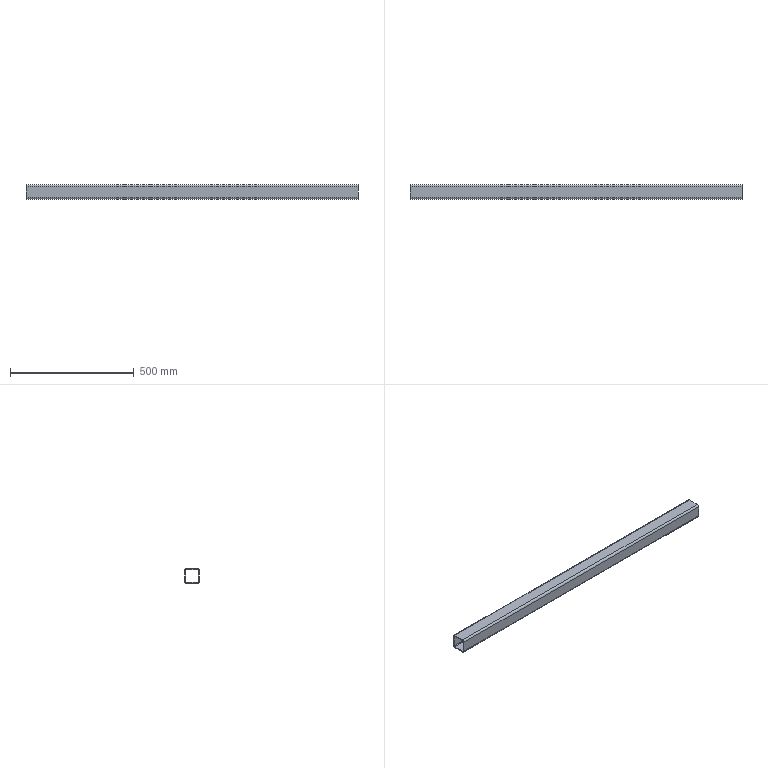Part | SolidWorks | features BaseBody 1 | 1 solid | 18 faces | box 1340 x 60 x 60 mm | volume 1145427 mm3 | plane 10 | cylinder 8 | commonest cylinder face diameters 8 x4 16 x4
STEP:
#1=CARTESIAN_POINT('',(-640.,44.,504.));
#2=VERTEX_POINT('',#1);
#3=CARTESIAN_POINT('',(-640.,0.,504.));
#4=VERTEX_POINT('',#3);
#5=CARTESIAN_POINT('',(-640.,44.,504.));
#6=DIRECTION('',(0.,-1.,0.));
#7=VECTOR('',#6,1000.);
#8=LINE('',#5,#7);
#9=EDGE_CURVE('',#2,#4,#8,.T.);
#10=ORIENTED_EDGE('',*,*,#9,.T.);
#11=CARTESIAN_POINT('',(700.,0.,504.));
#12=VERTEX_POINT('',#11);
#13=CARTESIAN_POINT('',(-670.,0.,504.));
#14=DIRECTION('',(1.,0.,0.));
#15=VECTOR('',#14,1000.);
#16=LINE('',#13,#15);
#17=EDGE_CURVE('',#4,#12,#16,.T.);
#18=ORIENTED_EDGE('',*,*,#17,.T.);
#19=CARTESIAN_POINT('',(700.,44.,504.));
#20=VERTEX_POINT('',#19);
#21=CARTESIAN_POINT('',(700.,44.,504.));
#22=DIRECTION('',(0.,1.,0.));
#23=VECTOR('',#22,1000.);
#24=LINE('',#21,#23);
#25=EDGE_CURVE('',#12,#20,#24,.T.);
#26=ORIENTED_EDGE('',*,*,#25,.T.);
#27=CARTESIAN_POINT('',(-670.,44.,504.));
#28=DIRECTION('',(-1.,0.,0.));
#29=VECTOR('',#28,1000.);
#30=LINE('',#27,#29);
#31=EDGE_CURVE('',#20,#2,#30,.T.);
#32=ORIENTED_EDGE('',*,*,#31,.T.);
#33=EDGE_LOOP('',(#10,#18,#26,#32));
#34=FACE_OUTER_BOUND('',#33,.T.);
#35=CARTESIAN_POINT('',(-670.,44.,504.));
#36=DIRECTION('',(0.,0.,1.));
#37=DIRECTION('',(1.,0.,0.));
#38=AXIS2_PLACEMENT_3D('',#35,#36,#37);
#39=PLANE('',#38);
#40=ADVANCED_FACE('',(#34),#39,.T.);
#41=ORIENTED_EDGE('',*,*,#17,.F.);
#42=CARTESIAN_POINT('',(-640.,-4.,508.));
#43=VERTEX_POINT('',#42);
#44=CARTESIAN_POINT('',(-640.,0.,508.));
#45=DIRECTION('',(1.,0.,0.));
#46=DIRECTION('',(0.,0.,-1.));
#47=AXIS2_PLACEMENT_3D('',#44,#45,#46);
#48=CIRCLE('',#47,4.);
#49=EDGE_CURVE('',#43,#4,#48,.T.);
#50=ORIENTED_EDGE('',*,*,#49,.F.);
#51=CARTESIAN_POINT('',(700.,-4.,508.));
#52=VERTEX_POINT('',#51);
#53=CARTESIAN_POINT('',(-670.,-4.,508.));
#54=DIRECTION('',(-1.,0.,0.));
#55=VECTOR('',#54,1000.);
#56=LINE('',#53,#55);
#57=EDGE_CURVE('',#52,#43,#56,.T.);
#58=ORIENTED_EDGE('',*,*,#57,.F.);
#59=CARTESIAN_POINT('',(700.,0.,508.));
#60=DIRECTION('',(-1.,0.,0.));
#61=DIRECTION('',(0.,0.,-1.));
#62=AXIS2_PLACEMENT_3D('',#59,#60,#61);
#63=CIRCLE('',#62,4.);
#64=EDGE_CURVE('',#12,#52,#63,.T.);
#65=ORIENTED_EDGE('',*,*,#64,.F.);
#66=EDGE_LOOP('',(#41,#50,#58,#65));
#67=FACE_OUTER_BOUND('',#66,.T.);
#68=CARTESIAN_POINT('',(-670.,0.,508.));
#69=DIRECTION('',(1.,0.,0.));
#70=DIRECTION('',(0.,0.,-1.));
#71=AXIS2_PLACEMENT_3D('',#68,#69,#70);
#72=CYLINDRICAL_SURFACE('',#71,4.);
#73=ADVANCED_FACE('',(#67),#72,.F.);
#74=ORIENTED_EDGE('',*,*,#49,.T.);
#75=ORIENTED_EDGE('',*,*,#9,.F.);
#76=CARTESIAN_POINT('',(-640.,48.,508.));
#77=VERTEX_POINT('',#76);
#78=CARTESIAN_POINT('',(-640.,44.,508.));
#79=DIRECTION('',(1.,0.,0.));
#80=DIRECTION('',(0.,0.,-1.));
#81=AXIS2_PLACEMENT_3D('',#78,#79,#80);
#82=CIRCLE('',#81,4.);
#83=EDGE_CURVE('',#2,#77,#82,.T.);
#84=ORIENTED_EDGE('',*,*,#83,.T.);
#85=CARTESIAN_POINT('',(-640.,48.,552.));
#86=VERTEX_POINT('',#85);
#87=CARTESIAN_POINT('',(-640.,48.,508.));
#88=DIRECTION('',(0.,0.,1.));
#89=VECTOR('',#88,1000.);
#90=LINE('',#87,#89);
#91=EDGE_CURVE('',#77,#86,#90,.T.);
#92=ORIENTED_EDGE('',*,*,#91,.T.);
#93=CARTESIAN_POINT('',(-640.,44.,556.));
#94=VERTEX_POINT('',#93);
#95=CARTESIAN_POINT('',(-640.,44.,552.));
#96=DIRECTION('',(1.,0.,0.));
#97=DIRECTION('',(0.,0.,-1.));
#98=AXIS2_PLACEMENT_3D('',#95,#96,#97);
#99=CIRCLE('',#98,4.);
#100=EDGE_CURVE('',#86,#94,#99,.T.);
#101=ORIENTED_EDGE('',*,*,#100,.T.);
#102=CARTESIAN_POINT('',(-640.,0.,556.));
#103=VERTEX_POINT('',#102);
#104=CARTESIAN_POINT('',(-640.,1242.,556.));
#105=DIRECTION('',(0.,-1.,0.));
#106=VECTOR('',#105,1000.);
#107=LINE('',#104,#106);
#108=EDGE_CURVE('',#94,#103,#107,.T.);
#109=ORIENTED_EDGE('',*,*,#108,.T.);
#110=CARTESIAN_POINT('',(-640.,-4.,552.));
#111=VERTEX_POINT('',#110);
#112=CARTESIAN_POINT('',(-640.,0.,552.));
#113=DIRECTION('',(1.,0.,0.));
#114=DIRECTION('',(0.,0.,-1.));
#115=AXIS2_PLACEMENT_3D('',#112,#113,#114);
#116=CIRCLE('',#115,4.);
#117=EDGE_CURVE('',#103,#111,#116,.T.);
#118=ORIENTED_EDGE('',*,*,#117,.T.);
#119=CARTESIAN_POINT('',(-640.,-4.,508.));
#120=DIRECTION('',(0.,0.,-1.));
#121=VECTOR('',#120,1000.);
#122=LINE('',#119,#121);
#123=EDGE_CURVE('',#111,#43,#122,.T.);
#124=ORIENTED_EDGE('',*,*,#123,.T.);
#125=EDGE_LOOP('',(#74,#75,#84,#92,#101,#109,#118,#124));
#126=FACE_BOUND('',#125,.T.);
#127=CARTESIAN_POINT('',(-640.,44.,500.));
#128=VERTEX_POINT('',#127);
#129=CARTESIAN_POINT('',(-640.,0.,500.));
#130=VERTEX_POINT('',#129);
#131=CARTESIAN_POINT('',(-640.,1242.,500.));
#132=DIRECTION('',(0.,-1.,0.));
#133=VECTOR('',#132,1000.);
#134=LINE('',#131,#133);
#135=EDGE_CURVE('',#128,#130,#134,.T.);
#136=ORIENTED_EDGE('',*,*,#135,.T.);
#137=CARTESIAN_POINT('',(-640.,-8.,508.));
#138=VERTEX_POINT('',#137);
#139=CARTESIAN_POINT('',(-640.,0.,508.));
#140=DIRECTION('',(-1.,0.,0.));
#141=DIRECTION('',(0.,0.,-1.));
#142=AXIS2_PLACEMENT_3D('',#139,#140,#141);
#143=CIRCLE('',#142,8.);
#144=EDGE_CURVE('',#130,#138,#143,.T.);
#145=ORIENTED_EDGE('',*,*,#144,.T.);
#146=CARTESIAN_POINT('',(-640.,-8.,552.));
#147=VERTEX_POINT('',#146);
#148=CARTESIAN_POINT('',(-640.,-8.,508.));
#149=DIRECTION('',(0.,0.,1.));
#150=VECTOR('',#149,1000.);
#151=LINE('',#148,#150);
#152=EDGE_CURVE('',#138,#147,#151,.T.);
#153=ORIENTED_EDGE('',*,*,#152,.T.);
#154=CARTESIAN_POINT('',(-640.,0.,560.));
#155=VERTEX_POINT('',#154);
#156=CARTESIAN_POINT('',(-640.,0.,552.));
#157=DIRECTION('',(-1.,0.,0.));
#158=DIRECTION('',(0.,0.,-1.));
#159=AXIS2_PLACEMENT_3D('',#156,#157,#158);
#160=CIRCLE('',#159,8.);
#161=EDGE_CURVE('',#147,#155,#160,.T.);
#162=ORIENTED_EDGE('',*,*,#161,.T.);
#163=CARTESIAN_POINT('',(-640.,44.,560.));
#164=VERTEX_POINT('',#163);
#165=CARTESIAN_POINT('',(-640.,1242.,560.));
#166=DIRECTION('',(0.,1.,0.));
#167=VECTOR('',#166,1000.);
#168=LINE('',#165,#167);
#169=EDGE_CURVE('',#155,#164,#168,.T.);
#170=ORIENTED_EDGE('',*,*,#169,.T.);
#171=CARTESIAN_POINT('',(-640.,52.,552.));
#172=VERTEX_POINT('',#171);
#173=CARTESIAN_POINT('',(-640.,44.,552.));
#174=DIRECTION('',(-1.,0.,0.));
#175=DIRECTION('',(0.,0.,-1.));
#176=AXIS2_PLACEMENT_3D('',#173,#174,#175);
#177=CIRCLE('',#176,8.);
#178=EDGE_CURVE('',#164,#172,#177,.T.);
#179=ORIENTED_EDGE('',*,*,#178,.T.);
#180=CARTESIAN_POINT('',(-640.,52.,508.));
#181=VERTEX_POINT('',#180);
#182=CARTESIAN_POINT('',(-640.,52.,508.));
#183=DIRECTION('',(0.,0.,-1.));
#184=VECTOR('',#183,1000.);
#185=LINE('',#182,#184);
#186=EDGE_CURVE('',#172,#181,#185,.T.);
#187=ORIENTED_EDGE('',*,*,#186,.T.);
#188=CARTESIAN_POINT('',(-640.,44.,508.));
#189=DIRECTION('',(-1.,0.,0.));
#190=DIRECTION('',(0.,0.,-1.));
#191=AXIS2_PLACEMENT_3D('',#188,#189,#190);
#192=CIRCLE('',#191,8.);
#193=EDGE_CURVE('',#181,#128,#192,.T.);
#194=ORIENTED_EDGE('',*,*,#193,.T.);
#195=EDGE_LOOP('',(#136,#145,#153,#162,#170,#179,#187,#194));
#196=FACE_OUTER_BOUND('',#195,.T.);
#197=CARTESIAN_POINT('',(-640.,1242.,508.));
#198=DIRECTION('',(-1.,0.,0.));
#199=DIRECTION('',(0.,0.,1.));
#200=AXIS2_PLACEMENT_3D('',#197,#198,#199);
#201=PLANE('',#200);
#202=ADVANCED_FACE('',(#126,#196),#201,.T.);
#203=CARTESIAN_POINT('',(700.,48.,508.));
#204=VERTEX_POINT('',#203);
#205=CARTESIAN_POINT('',(-670.,48.,508.));
#206=DIRECTION('',(1.,0.,0.));
#207=VECTOR('',#206,1000.);
#208=LINE('',#205,#207);
#209=EDGE_CURVE('',#77,#204,#208,.T.);
#210=ORIENTED_EDGE('',*,*,#209,.F.);
#211=ORIENTED_EDGE('',*,*,#83,.F.);
#212=ORIENTED_EDGE('',*,*,#31,.F.);
#213=CARTESIAN_POINT('',(700.,44.,508.));
#214=DIRECTION('',(-1.,0.,0.));
#215=DIRECTION('',(0.,0.,-1.));
#216=AXIS2_PLACEMENT_3D('',#213,#214,#215);
#217=CIRCLE('',#216,4.);
#218=EDGE_CURVE('',#204,#20,#217,.T.);
#219=ORIENTED_EDGE('',*,*,#218,.F.);
#220=EDGE_LOOP('',(#210,#211,#212,#219));
#221=FACE_OUTER_BOUND('',#220,.T.);
#222=CARTESIAN_POINT('',(-670.,44.,508.));
#223=DIRECTION('',(1.,0.,0.));
#224=DIRECTION('',(0.,0.,-1.));
#225=AXIS2_PLACEMENT_3D('',#222,#223,#224);
#226=CYLINDRICAL_SURFACE('',#225,4.);
#227=ADVANCED_FACE('',(#221),#226,.F.);
#228=ORIENTED_EDGE('',*,*,#25,.F.);
#229=ORIENTED_EDGE('',*,*,#64,.T.);
#230=CARTESIAN_POINT('',(700.,-4.,552.));
#231=VERTEX_POINT('',#230);
#232=CARTESIAN_POINT('',(700.,-4.,530.));
#233=DIRECTION('',(0.,0.,1.));
#234=VECTOR('',#233,1000.);
#235=LINE('',#232,#234);
#236=EDGE_CURVE('',#52,#231,#235,.T.);
#237=ORIENTED_EDGE('',*,*,#236,.T.);
#238=CARTESIAN_POINT('',(700.,0.,556.));
#239=VERTEX_POINT('',#238);
#240=CARTESIAN_POINT('',(700.,0.,552.));
#241=DIRECTION('',(-1.,0.,0.));
#242=DIRECTION('',(0.,0.,-1.));
#243=AXIS2_PLACEMENT_3D('',#240,#241,#242);
#244=CIRCLE('',#243,4.);
#245=EDGE_CURVE('',#231,#239,#244,.T.);
#246=ORIENTED_EDGE('',*,*,#245,.T.);
#247=CARTESIAN_POINT('',(700.,44.,556.));
#248=VERTEX_POINT('',#247);
#249=CARTESIAN_POINT('',(700.,52.,556.));
#250=DIRECTION('',(0.,1.,0.));
#251=VECTOR('',#250,1000.);
#252=LINE('',#249,#251);
#253=EDGE_CURVE('',#239,#248,#252,.T.);
#254=ORIENTED_EDGE('',*,*,#253,.T.);
#255=CARTESIAN_POINT('',(700.,48.,552.));
#256=VERTEX_POINT('',#255);
#257=CARTESIAN_POINT('',(700.,44.,552.));
#258=DIRECTION('',(-1.,0.,0.));
#259=DIRECTION('',(0.,0.,-1.));
#260=AXIS2_PLACEMENT_3D('',#257,#258,#259);
#261=CIRCLE('',#260,4.);
#262=EDGE_CURVE('',#248,#256,#261,.T.);
#263=ORIENTED_EDGE('',*,*,#262,.T.);
#264=CARTESIAN_POINT('',(700.,48.,530.));
#265=DIRECTION('',(0.,0.,-1.));
#266=VECTOR('',#265,1000.);
#267=LINE('',#264,#266);
#268=EDGE_CURVE('',#256,#204,#267,.T.);
#269=ORIENTED_EDGE('',*,*,#268,.T.);
#270=ORIENTED_EDGE('',*,*,#218,.T.);
#271=EDGE_LOOP('',(#228,#229,#237,#246,#254,#263,#269,#270));
#272=FACE_BOUND('',#271,.T.);
#273=CARTESIAN_POINT('',(700.,-8.,508.));
#274=VERTEX_POINT('',#273);
#275=CARTESIAN_POINT('',(700.,0.,500.));
#276=VERTEX_POINT('',#275);
#277=CARTESIAN_POINT('',(700.,0.,508.));
#278=DIRECTION('',(1.,0.,0.));
#279=DIRECTION('',(0.,0.,-1.));
#280=AXIS2_PLACEMENT_3D('',#277,#278,#279);
#281=CIRCLE('',#280,8.);
#282=EDGE_CURVE('',#274,#276,#281,.T.);
#283=ORIENTED_EDGE('',*,*,#282,.T.);
#284=CARTESIAN_POINT('',(700.,44.,500.));
#285=VERTEX_POINT('',#284);
#286=CARTESIAN_POINT('',(700.,52.,500.));
#287=DIRECTION('',(0.,1.,0.));
#288=VECTOR('',#287,1000.);
#289=LINE('',#286,#288);
#290=EDGE_CURVE('',#276,#285,#289,.T.);
#291=ORIENTED_EDGE('',*,*,#290,.T.);
#292=CARTESIAN_POINT('',(700.,52.,508.));
#293=VERTEX_POINT('',#292);
#294=CARTESIAN_POINT('',(700.,44.,508.));
#295=DIRECTION('',(1.,0.,0.));
#296=DIRECTION('',(0.,0.,-1.));
#297=AXIS2_PLACEMENT_3D('',#294,#295,#296);
#298=CIRCLE('',#297,8.);
#299=EDGE_CURVE('',#285,#293,#298,.T.);
#300=ORIENTED_EDGE('',*,*,#299,.T.);
#301=CARTESIAN_POINT('',(700.,52.,552.));
#302=VERTEX_POINT('',#301);
#303=CARTESIAN_POINT('',(700.,52.,530.));
#304=DIRECTION('',(0.,0.,1.));
#305=VECTOR('',#304,1000.);
#306=LINE('',#303,#305);
#307=EDGE_CURVE('',#293,#302,#306,.T.);
#308=ORIENTED_EDGE('',*,*,#307,.T.);
#309=CARTESIAN_POINT('',(700.,44.,560.));
#310=VERTEX_POINT('',#309);
#311=CARTESIAN_POINT('',(700.,44.,552.));
#312=DIRECTION('',(1.,0.,0.));
#313=DIRECTION('',(0.,0.,-1.));
#314=AXIS2_PLACEMENT_3D('',#311,#312,#313);
#315=CIRCLE('',#314,8.);
#316=EDGE_CURVE('',#302,#310,#315,.T.);
#317=ORIENTED_EDGE('',*,*,#316,.T.);
#318=CARTESIAN_POINT('',(700.,0.,560.));
#319=VERTEX_POINT('',#318);
#320=CARTESIAN_POINT('',(700.,52.,560.));
#321=DIRECTION('',(0.,-1.,0.));
#322=VECTOR('',#321,1000.);
#323=LINE('',#320,#322);
#324=EDGE_CURVE('',#310,#319,#323,.T.);
#325=ORIENTED_EDGE('',*,*,#324,.T.);
#326=CARTESIAN_POINT('',(700.,-8.,552.));
#327=VERTEX_POINT('',#326);
#328=CARTESIAN_POINT('',(700.,0.,552.));
#329=DIRECTION('',(1.,0.,0.));
#330=DIRECTION('',(0.,0.,-1.));
#331=AXIS2_PLACEMENT_3D('',#328,#329,#330);
#332=CIRCLE('',#331,8.);
#333=EDGE_CURVE('',#319,#327,#332,.T.);
#334=ORIENTED_EDGE('',*,*,#333,.T.);
#335=CARTESIAN_POINT('',(700.,-8.,530.));
#336=DIRECTION('',(0.,0.,-1.));
#337=VECTOR('',#336,1000.);
#338=LINE('',#335,#337);
#339=EDGE_CURVE('',#327,#274,#338,.T.);
#340=ORIENTED_EDGE('',*,*,#339,.T.);
#341=EDGE_LOOP('',(#283,#291,#300,#308,#317,#325,#334,#340));
#342=FACE_OUTER_BOUND('',#341,.T.);
#343=CARTESIAN_POINT('',(700.,52.,530.));
#344=DIRECTION('',(1.,0.,0.));
#345=DIRECTION('',(0.,0.,-1.));
#346=AXIS2_PLACEMENT_3D('',#343,#344,#345);
#347=PLANE('',#346);
#348=ADVANCED_FACE('',(#272,#342),#347,.T.);
#349=ORIENTED_EDGE('',*,*,#123,.F.);
#350=CARTESIAN_POINT('',(-670.,-4.,552.));
#351=DIRECTION('',(1.,0.,0.));
#352=VECTOR('',#351,1000.);
#353=LINE('',#350,#352);
#354=EDGE_CURVE('',#111,#231,#353,.T.);
#355=ORIENTED_EDGE('',*,*,#354,.T.);
#356=ORIENTED_EDGE('',*,*,#236,.F.);
#357=ORIENTED_EDGE('',*,*,#57,.T.);
#358=EDGE_LOOP('',(#349,#355,#356,#357));
#359=FACE_OUTER_BOUND('',#358,.T.);
#360=CARTESIAN_POINT('',(-670.,-4.,552.));
#361=DIRECTION('',(0.,1.,0.));
#362=DIRECTION('',(0.,0.,1.));
#363=AXIS2_PLACEMENT_3D('',#360,#361,#362);
#364=PLANE('',#363);
#365=ADVANCED_FACE('',(#359),#364,.T.);
#366=ORIENTED_EDGE('',*,*,#354,.F.);
#367=ORIENTED_EDGE('',*,*,#117,.F.);
#368=CARTESIAN_POINT('',(-670.,0.,556.));
#369=DIRECTION('',(-1.,0.,0.));
#370=VECTOR('',#369,1000.);
#371=LINE('',#368,#370);
#372=EDGE_CURVE('',#239,#103,#371,.T.);
#373=ORIENTED_EDGE('',*,*,#372,.F.);
#374=ORIENTED_EDGE('',*,*,#245,.F.);
#375=EDGE_LOOP('',(#366,#367,#373,#374));
#376=FACE_OUTER_BOUND('',#375,.T.);
#377=CARTESIAN_POINT('',(-670.,0.,552.));
#378=DIRECTION('',(1.,0.,0.));
#379=DIRECTION('',(0.,0.,-1.));
#380=AXIS2_PLACEMENT_3D('',#377,#378,#379);
#381=CYLINDRICAL_SURFACE('',#380,4.);
#382=ADVANCED_FACE('',(#376),#381,.F.);
#383=ORIENTED_EDGE('',*,*,#108,.F.);
#384=CARTESIAN_POINT('',(-670.,44.,556.));
#385=DIRECTION('',(1.,0.,0.));
#386=VECTOR('',#385,1000.);
#387=LINE('',#384,#386);
#388=EDGE_CURVE('',#94,#248,#387,.T.);
#389=ORIENTED_EDGE('',*,*,#388,.T.);
#390=ORIENTED_EDGE('',*,*,#253,.F.);
#391=ORIENTED_EDGE('',*,*,#372,.T.);
#392=EDGE_LOOP('',(#383,#389,#390,#391));
#393=FACE_OUTER_BOUND('',#392,.T.);
#394=CARTESIAN_POINT('',(-670.,0.,556.));
#395=DIRECTION('',(0.,0.,-1.));
#396=DIRECTION('',(-1.,0.,0.));
#397=AXIS2_PLACEMENT_3D('',#394,#395,#396);
#398=PLANE('',#397);
#399=ADVANCED_FACE('',(#393),#398,.T.);
#400=ORIENTED_EDGE('',*,*,#388,.F.);
#401=ORIENTED_EDGE('',*,*,#100,.F.);
#402=CARTESIAN_POINT('',(-670.,48.,552.));
#403=DIRECTION('',(-1.,0.,0.));
#404=VECTOR('',#403,1000.);
#405=LINE('',#402,#404);
#406=EDGE_CURVE('',#256,#86,#405,.T.);
#407=ORIENTED_EDGE('',*,*,#406,.F.);
#408=ORIENTED_EDGE('',*,*,#262,.F.);
#409=EDGE_LOOP('',(#400,#401,#407,#408));
#410=FACE_OUTER_BOUND('',#409,.T.);
#411=CARTESIAN_POINT('',(-670.,44.,552.));
#412=DIRECTION('',(1.,0.,0.));
#413=DIRECTION('',(0.,0.,-1.));
#414=AXIS2_PLACEMENT_3D('',#411,#412,#413);
#415=CYLINDRICAL_SURFACE('',#414,4.);
#416=ADVANCED_FACE('',(#410),#415,.F.);
#417=ORIENTED_EDGE('',*,*,#91,.F.);
#418=ORIENTED_EDGE('',*,*,#209,.T.);
#419=ORIENTED_EDGE('',*,*,#268,.F.);
#420=ORIENTED_EDGE('',*,*,#406,.T.);
#421=EDGE_LOOP('',(#417,#418,#419,#420));
#422=FACE_OUTER_BOUND('',#421,.T.);
#423=CARTESIAN_POINT('',(-670.,48.,508.));
#424=DIRECTION('',(0.,-1.,0.));
#425=DIRECTION('',(0.,0.,-1.));
#426=AXIS2_PLACEMENT_3D('',#423,#424,#425);
#427=PLANE('',#426);
#428=ADVANCED_FACE('',(#422),#427,.T.);
#429=CARTESIAN_POINT('',(-670.,0.,500.));
#430=DIRECTION('',(1.,0.,0.));
#431=VECTOR('',#430,1000.);
#432=LINE('',#429,#431);
#433=EDGE_CURVE('',#130,#276,#432,.T.);
#434=ORIENTED_EDGE('',*,*,#433,.T.);
#435=ORIENTED_EDGE('',*,*,#282,.F.);
#436=CARTESIAN_POINT('',(-670.,-8.,508.));
#437=DIRECTION('',(-1.,0.,0.));
#438=VECTOR('',#437,1000.);
#439=LINE('',#436,#438);
#440=EDGE_CURVE('',#274,#138,#439,.T.);
#441=ORIENTED_EDGE('',*,*,#440,.T.);
#442=ORIENTED_EDGE('',*,*,#144,.F.);
#443=EDGE_LOOP('',(#434,#435,#441,#442));
#444=FACE_OUTER_BOUND('',#443,.T.);
#445=CARTESIAN_POINT('',(-670.,0.,508.));
#446=DIRECTION('',(1.,0.,0.));
#447=DIRECTION('',(0.,0.,-1.));
#448=AXIS2_PLACEMENT_3D('',#445,#446,#447);
#449=CYLINDRICAL_SURFACE('',#448,8.);
#450=ADVANCED_FACE('',(#444),#449,.T.);
#451=ORIENTED_EDGE('',*,*,#135,.F.);
#452=CARTESIAN_POINT('',(-670.,44.,500.));
#453=DIRECTION('',(-1.,0.,0.));
#454=VECTOR('',#453,1000.);
#455=LINE('',#452,#454);
#456=EDGE_CURVE('',#285,#128,#455,.T.);
#457=ORIENTED_EDGE('',*,*,#456,.F.);
#458=ORIENTED_EDGE('',*,*,#290,.F.);
#459=ORIENTED_EDGE('',*,*,#433,.F.);
#460=EDGE_LOOP('',(#451,#457,#458,#459));
#461=FACE_OUTER_BOUND('',#460,.T.);
#462=CARTESIAN_POINT('',(-670.,44.,500.));
#463=DIRECTION('',(0.,0.,1.));
#464=DIRECTION('',(1.,0.,0.));
#465=AXIS2_PLACEMENT_3D('',#462,#463,#464);
#466=PLANE('',#465);
#467=ADVANCED_FACE('',(#461),#466,.F.);
#468=CARTESIAN_POINT('',(-670.,52.,508.));
#469=DIRECTION('',(1.,0.,0.));
#470=VECTOR('',#469,1000.);
#471=LINE('',#468,#470);
#472=EDGE_CURVE('',#181,#293,#471,.T.);
#473=ORIENTED_EDGE('',*,*,#472,.T.);
#474=ORIENTED_EDGE('',*,*,#299,.F.);
#475=ORIENTED_EDGE('',*,*,#456,.T.);
#476=ORIENTED_EDGE('',*,*,#193,.F.);
#477=EDGE_LOOP('',(#473,#474,#475,#476));
#478=FACE_OUTER_BOUND('',#477,.T.);
#479=CARTESIAN_POINT('',(-670.,44.,508.));
#480=DIRECTION('',(1.,0.,0.));
#481=DIRECTION('',(0.,0.,-1.));
#482=AXIS2_PLACEMENT_3D('',#479,#480,#481);
#483=CYLINDRICAL_SURFACE('',#482,8.);
#484=ADVANCED_FACE('',(#478),#483,.T.);
#485=ORIENTED_EDGE('',*,*,#186,.F.);
#486=CARTESIAN_POINT('',(-670.,52.,552.));
#487=DIRECTION('',(-1.,0.,0.));
#488=VECTOR('',#487,1000.);
#489=LINE('',#486,#488);
#490=EDGE_CURVE('',#302,#172,#489,.T.);
#491=ORIENTED_EDGE('',*,*,#490,.F.);
#492=ORIENTED_EDGE('',*,*,#307,.F.);
#493=ORIENTED_EDGE('',*,*,#472,.F.);
#494=EDGE_LOOP('',(#485,#491,#492,#493));
#495=FACE_OUTER_BOUND('',#494,.T.);
#496=CARTESIAN_POINT('',(-670.,52.,508.));
#497=DIRECTION('',(0.,-1.,0.));
#498=DIRECTION('',(0.,0.,-1.));
#499=AXIS2_PLACEMENT_3D('',#496,#497,#498);
#500=PLANE('',#499);
#501=ADVANCED_FACE('',(#495),#500,.F.);
#502=CARTESIAN_POINT('',(-670.,44.,560.));
#503=DIRECTION('',(1.,0.,0.));
#504=VECTOR('',#503,1000.);
#505=LINE('',#502,#504);
#506=EDGE_CURVE('',#164,#310,#505,.T.);
#507=ORIENTED_EDGE('',*,*,#506,.T.);
#508=ORIENTED_EDGE('',*,*,#316,.F.);
#509=ORIENTED_EDGE('',*,*,#490,.T.);
#510=ORIENTED_EDGE('',*,*,#178,.F.);
#511=EDGE_LOOP('',(#507,#508,#509,#510));
#512=FACE_OUTER_BOUND('',#511,.T.);
#513=CARTESIAN_POINT('',(-670.,44.,552.));
#514=DIRECTION('',(1.,0.,0.));
#515=DIRECTION('',(0.,0.,-1.));
#516=AXIS2_PLACEMENT_3D('',#513,#514,#515);
#517=CYLINDRICAL_SURFACE('',#516,8.);
#518=ADVANCED_FACE('',(#512),#517,.T.);
#519=ORIENTED_EDGE('',*,*,#169,.F.);
#520=CARTESIAN_POINT('',(-670.,0.,560.));
#521=DIRECTION('',(-1.,0.,0.));
#522=VECTOR('',#521,1000.);
#523=LINE('',#520,#522);
#524=EDGE_CURVE('',#319,#155,#523,.T.);
#525=ORIENTED_EDGE('',*,*,#524,.F.);
#526=ORIENTED_EDGE('',*,*,#324,.F.);
#527=ORIENTED_EDGE('',*,*,#506,.F.);
#528=EDGE_LOOP('',(#519,#525,#526,#527));
#529=FACE_OUTER_BOUND('',#528,.T.);
#530=CARTESIAN_POINT('',(-670.,0.,560.));
#531=DIRECTION('',(0.,0.,-1.));
#532=DIRECTION('',(-1.,0.,0.));
#533=AXIS2_PLACEMENT_3D('',#530,#531,#532);
#534=PLANE('',#533);
#535=ADVANCED_FACE('',(#529),#534,.F.);
#536=CARTESIAN_POINT('',(-670.,-8.,552.));
#537=DIRECTION('',(1.,0.,0.));
#538=VECTOR('',#537,1000.);
#539=LINE('',#536,#538);
#540=EDGE_CURVE('',#147,#327,#539,.T.);
#541=ORIENTED_EDGE('',*,*,#540,.T.);
#542=ORIENTED_EDGE('',*,*,#333,.F.);
#543=ORIENTED_EDGE('',*,*,#524,.T.);
#544=ORIENTED_EDGE('',*,*,#161,.F.);
#545=EDGE_LOOP('',(#541,#542,#543,#544));
#546=FACE_OUTER_BOUND('',#545,.T.);
#547=CARTESIAN_POINT('',(-670.,0.,552.));
#548=DIRECTION('',(1.,0.,0.));
#549=DIRECTION('',(0.,0.,-1.));
#550=AXIS2_PLACEMENT_3D('',#547,#548,#549);
#551=CYLINDRICAL_SURFACE('',#550,8.);
#552=ADVANCED_FACE('',(#546),#551,.T.);
#553=ORIENTED_EDGE('',*,*,#152,.F.);
#554=ORIENTED_EDGE('',*,*,#440,.F.);
#555=ORIENTED_EDGE('',*,*,#339,.F.);
#556=ORIENTED_EDGE('',*,*,#540,.F.);
#557=EDGE_LOOP('',(#553,#554,#555,#556));
#558=FACE_OUTER_BOUND('',#557,.T.);
#559=CARTESIAN_POINT('',(-670.,-8.,552.));
#560=DIRECTION('',(0.,1.,0.));
#561=DIRECTION('',(0.,0.,1.));
#562=AXIS2_PLACEMENT_3D('',#559,#560,#561);
#563=PLANE('',#562);
#564=ADVANCED_FACE('',(#558),#563,.F.);
#565=CLOSED_SHELL('',(#40,#73,#202,#227,#348,#365,#382,#399,#416,#428,#450,#467,#484,#501,#518,#535,#552,#564));
#566=MANIFOLD_SOLID_BREP('',#565);
#567=CARTESIAN_POINT('',(0.,0.,0.));
#568=DIRECTION('',(0.,0.,1.));
#569=DIRECTION('',(1.,0.,0.));
#570=AXIS2_PLACEMENT_3D('',#567,#568,#569);
#571=(LENGTH_UNIT()NAMED_UNIT(*)SI_UNIT(.MILLI.,.METRE.));
#572=UNCERTAINTY_MEASURE_WITH_UNIT(LENGTH_MEASURE(0.00001),#571,'','');
#573=(NAMED_UNIT(*)PLANE_ANGLE_UNIT()SI_UNIT($,.RADIAN.));
#574=(NAMED_UNIT(*)SI_UNIT($,.STERADIAN.)SOLID_ANGLE_UNIT());
#575=(GEOMETRIC_REPRESENTATION_CONTEXT(3)GLOBAL_UNCERTAINTY_ASSIGNED_CONTEXT((#572))GLOBAL_UNIT_ASSIGNED_CONTEXT((#571,#573,#574))REPRESENTATION_CONTEXT('',''));
#576=ADVANCED_BREP_SHAPE_REPRESENTATION('',(#566,#570),#575);